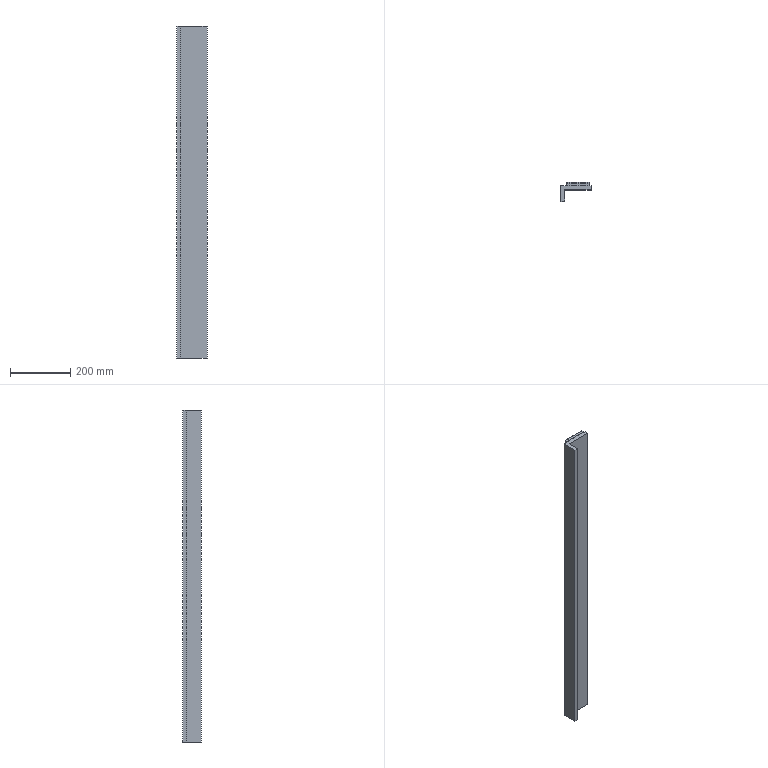Part | SolidWorks | features ICE 3, Extrusion 1, LPattern 1, MirrorPattern 1 | 1 solid | 116 faces | box 100 x 62 x 1100 mm | volume 2851141 mm3 | plane 116